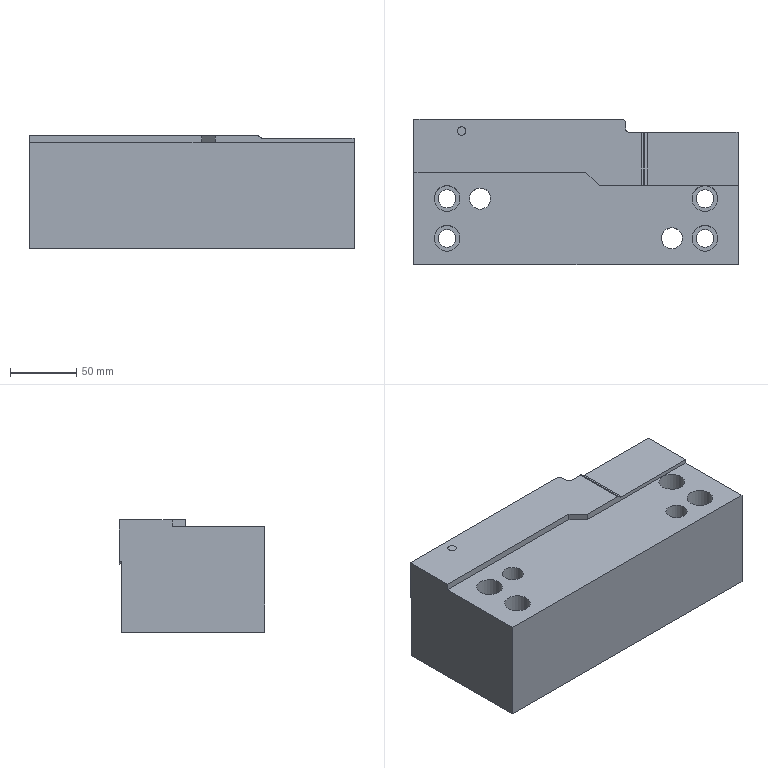Part | NX | features solid 2 | 1 solid | 35 faces | box 245 x 110 x 85 mm | volume 1990914 mm3 | plane 14 | spline 11 | cylinder 10 | commonest cylinder face diameters 13.5 x4 19.5 x4 16 x2